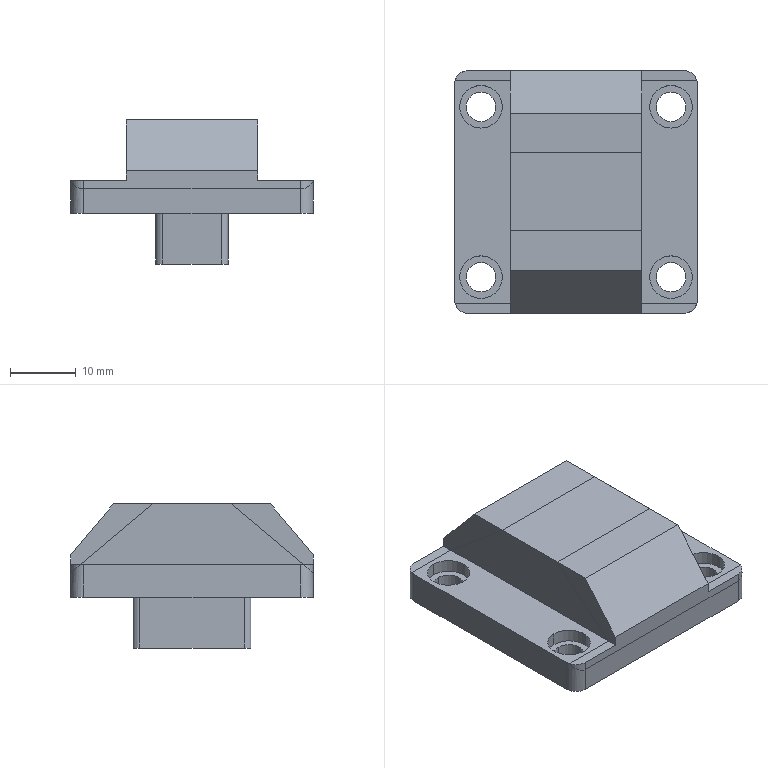CAM job | NX | 3+2 milling, drilling | part box 37 x 37 x 22 mm | stock box 43 x 43 x 25 mm
Tools:
number,name,description,diameter,corner_radius,flute_length,length,flutes
11,钻头5,Drilling Tool,6.0,0.0,35.0,50.0,2
10,G8-1,Thread Mill,7.7,0.0,10.0,50.0,3
9,钻头8.7,Drilling Tool,8.7,0.0,35.0,50.0,2
8,钻头6,Drilling Tool,6.0,0.0,35.0,50.0,2
5,钻头4.5,Drilling Tool,4.5,0.0,35.0,50.0,2
1,D50面刀,Milling Tool-5 Parameters,50.0,0.0,30.0,100.0,2
2,8C-20L-30L,Milling Tool-5 Parameters,8.0,0.0,20.0,65.0,2
3,8J-20L-30L,Milling Tool-5 Parameters,8.0,0.0,20.0,65.0,2
6,4C-10L-25L,Milling Tool-5 Parameters,4.0,0.0,10.0,65.0,2
4,D4点钻,Drilling Tool,4.0,0.0,10.0,75.0,2
7,D4R0.5,Milling Tool-5 Parameters,4.0,0.5,10.0,65.0,2
Operations:
program,operation,operation_type,tool,method,geometry_group,spindle_rpm,surface_speed,feed_per_tooth,feed_cut,feed_plunge,cut_length_mm,path_length_mm,cut_time_min,machine_time_min
A0101,FACE_MILLING,FaceMilling,D50面刀,METHOD,W1,3500.0,549.0,0.1143,800.0,100.0,126.0,160.0,0.1575,0.1609
A0101,ADAPTIVE_MILLING,CavityMilling,8C-20L-30L,METHOD,W1,5500.0,138.0,0.1818,2000.0,100.0,3052.006,3182.202,1.526,1.539
A0101,DRILLING,Operation,D4点钻,METHOD,W1,2500.0,31.0,0.05,250.0,0.0,14.0,205.708,0.056,0.0752
A0101,DRILLING_1,Operation,钻头4.5,METHOD,W1,2500.0,35.0,0.05,250.0,0.0,50.0,302.816,0.2,0.2253
A0101,HOLE_MILLING,CylinderMilling,4C-10L-25L,METHOD,W1,4500.0,56.0,0.0444,400.0,100.0,392.811,718.011,0.982,1.014
A0101,PLANAR_MILL,PlanarMilling,8J-20L-30L,METHOD,W1,4200.0,105.0,0.0952,800.0,100.0,223.86,566.11,0.2798,0.314
A0101,PLANAR_MILL_1,PlanarMilling,8J-20L-30L,METHOD,W1,4200.0,105.0,0.0952,800.0,100.0,353.686,418.186,0.4421,0.4486
A0101,PLANAR_MILL_2,PlanarMilling,D4点钻,METHOD,W1,4500.0,56.0,0.1111,1000.0,100.0,91.93,185.93,0.0919,0.1013
A0101,PLANAR_MILL_2_COPY,PlanarMilling,D4点钻,METHOD,W1,4500.0,56.0,0.1111,1000.0,100.0,92.884,239.264,0.0929,0.1075
A0101,PLANAR_MILL_3_COPY,PlanarMilling,D4点钻,METHOD,W1,4500.0,56.0,0.1111,1000.0,100.0,63.227,378.248,0.0632,0.0947
A0101,PLANAR_MILL_3,PlanarMilling,D4点钻,METHOD,W1,4500.0,56.0,0.1111,1000.0,100.0,87.415,387.454,0.0874,0.1174
A0101,ZLEVEL_PROFILE,ZLevelMilling,D4R0.5,METHOD,W1,5500.0,69.0,0.2273,2500.0,100.0,3162.345,3290.046,1.265,1.278
A0101,ZLEVEL_PROFILE_1,ZLevelMilling,D4R0.5,METHOD,MCS_1,5500.0,69.0,0.1364,1500.0,100.0,1234.218,1338.903,0.8228,0.8333
B0101,PLANAR_PROFILING,PlanarMilling,D50面刀,METHOD,W2,3500.0,549.0,0.1714,1200.0,100.0,637.0,846.8,0.5308,0.5518
B0101,PLANAR_PROFILING_COPY,PlanarMilling,D50面刀,METHOD,W2,3500.0,549.0,0.0857,600.0,100.0,91.0,127.0,0.1517,0.1553
B0101,DRILLING_2,Operation,D4点钻,METHOD,W2,2500.0,31.0,0.05,250.0,0.0,4.5,49.0,0.018,0.0224
B0101,DRILLING_4_COPY_1,Operation,钻头5,METHOD,W2,1600.0,30.0,0.0625,200.0,0.0,22.303,84.605,0.1115,0.1177
B0101,DRILLING_4,Operation,钻头6,METHOD,W2,1600.0,30.0,0.0625,200.0,0.0,22.303,84.605,0.1115,0.1177
B0101,DRILLING_3,Operation,钻头8.7,METHOD,W2,1600.0,30.0,0.0625,200.0,0.0,14.364,68.728,0.0718,0.0773
B0101,PLANAR_MILL_4,PlanarMilling,D4点钻,METHOD,W2,4500.0,56.0,0.0889,800.0,100.0,30.941,67.941,0.0387,0.0424
B0101,THREAD_MILLING,ThreadMilling,G8-1,METHOD,W2,4500.0,108.0,0.0148,200.0,100.0,93.067,421.807,0.4653,0.4982
G56,PLANAR_PROFILING_1,PlanarMilling,D50面刀,METHOD,W3,3500.0,549.0,0.1714,1200.0,100.0,637.0,846.8,0.5308,0.5518
G56,PLANAR_PROFILING_1_COPY,PlanarMilling,D50面刀,METHOD,W3,3500.0,549.0,0.1143,800.0,100.0,91.0,127.0,0.1138,0.1174
G56,DRILLING_2_COPY,Operation,D4点钻,METHOD,W3,2500.0,31.0,0.05,250.0,0.0,4.5,49.0,0.018,0.0225
G56,DRILLING_4_COPY_COPY,Operation,钻头5,METHOD,W3,1600.0,30.0,0.0625,200.0,0.0,23.303,86.605,0.1165,0.1228
G56,DRILLING_4_COPY,Operation,钻头6,METHOD,W3,1600.0,30.0,0.0625,200.0,0.0,23.303,86.605,0.1165,0.1228
G56,DRILLING_3_COPY,Operation,钻头8.7,METHOD,W3,1600.0,30.0,0.0625,200.0,0.0,14.364,68.728,0.0718,0.0773
G56,PLANAR_MILL_4_COPY,PlanarMilling,D4点钻,METHOD,W3,4500.0,56.0,0.0889,800.0,100.0,30.941,67.941,0.0387,0.0424
G56,THREAD_MILLING_COPY,ThreadMilling,G8-1,METHOD,W3,4500.0,108.0,0.0148,200.0,100.0,93.067,421.807,0.4653,0.4982
G57,FACE_MILLING_2,FaceMilling,D50面刀,METHOD,W4,4500.0,706.0,0.1333,1200.0,100.0,468.0,924.5,0.39,0.4356
G57,FACE_MILLING_2_COPY,FaceMilling,D50面刀,METHOD,W4,4500.0,706.0,0.0889,800.0,100.0,117.0,151.0,0.1462,0.1496
G57,ADAPTIVE_MILLING_1,CavityMilling,8C-20L-30L,METHOD,W4,5500.0,138.0,0.2273,2500.0,100.0,2301.593,2350.893,0.9206,0.9256
G57,FACE_MILLING_3,FaceMilling,8J-20L-30L,METHOD,W4,4500.0,113.0,0.0889,800.0,100.0,538.312,587.812,0.6729,0.6778
G57,PLANAR_MILL_5,PlanarMilling,D4点钻,METHOD,W4,3500.0,43.0,0.1143,800.0,100.0,76.737,113.737,0.0959,0.0996
G57,PLANAR_MILL_5_COPY,PlanarMilling,D4点钻,METHOD,W4,3500.0,43.0,0.1143,800.0,100.0,165.041,217.541,0.2063,0.2116
G57,PLANAR_MILL_5_COPY_COPY,PlanarMilling,D4点钻,METHOD,W4,3500.0,43.0,0.1143,800.0,100.0,46.62,340.019,0.0583,0.0876